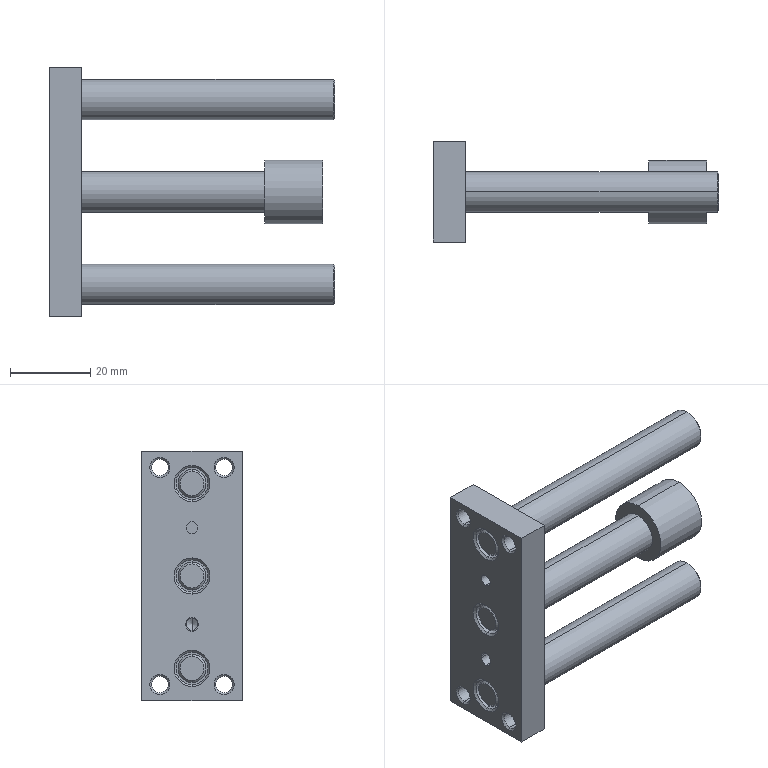Part | STEP file | 11-_TCM-16x25-0_25fp11 | 1 solid | 90 faces | box 71 x 25 x 62 mm | volume 28003 mm3 | cylinder 35 | cone 34 | plane 21 | commonest cylinder face diameters 4.134 x8 3 x7 7 x6 8 x6 10 x6 15.9 x2